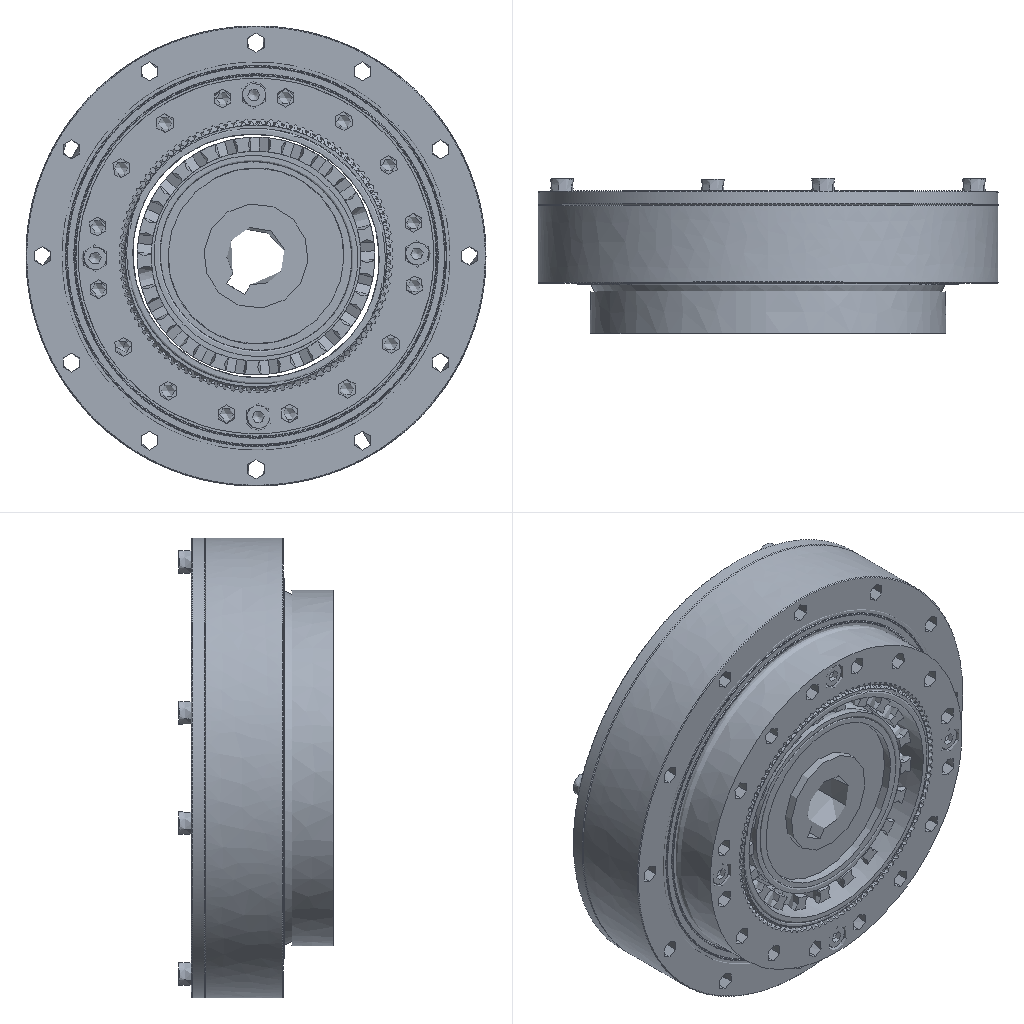Simulation study | ansys workbench
Set-up summary:
category,name,step,type,value,unit,region
solver,ansys_mapdl
solver,version,,,22.1
units,MPA,,stated
analysis,deck,,transient,transient
load_step,requested,,,1
analysis,nlgeom,,,True
mesh,nodes,,,225226
mesh,elements,,,154411
element_type,ANSYS 187 (type 1),,solid,2128
element_type,ANSYS 187 (type 2),,solid,3188
element_type,ANSYS 187 (type 3),,solid,1342
element_type,ANSYS 187 (type 4),,solid,24713
element_type,ANSYS 187 (type 5),,solid,9653
element_type,ANSYS 187 (type 6),,solid,9049
element_type,ANSYS 187 (type 7),,solid,3636
element_type,ANSYS 187 (type 8),,solid,2693
element_type,ANSYS 187 (type 9),,solid,23046
element_type,ANSYS 187 (type 10),,solid,29778
element_type,ANSYS 187 (type 11),,solid,1220
element_type,ANSYS 187 (type 12),,solid,1220
element_type,ANSYS 187 (type 13),,solid,1220
element_type,ANSYS 187 (type 14),,solid,1220
element_type,ANSYS 187 (type 15),,solid,1220
element_type,ANSYS 187 (type 16),,solid,1220
element_type,ANSYS 187 (type 17),,solid,1220
element_type,ANSYS 187 (type 18),,solid,1220
element_type,ANSYS 174 (type 19),,contact,1577
element_type,ANSYS 170 (type 20),,target,1577
element_type,ANSYS 174 (type 21),,contact,2406
element_type,ANSYS 170 (type 22),,target,2406
element_type,ANSYS 174 (type 23),,contact,561
element_type,ANSYS 170 (type 24),,target,561
element_type,ANSYS 174 (type 25),,contact,396
element_type,ANSYS 170 (type 26),,target,396
element_type,ANSYS 174 (type 27),,contact,1694
element_type,ANSYS 170 (type 28),,target,1694
element_type,ANSYS 174 (type 29),,contact,3067
element_type,ANSYS 170 (type 30),,target,3067
element_type,ANSYS 174 (type 31),,contact,124
element_type,ANSYS 170 (type 32),,target,124
element_type,ANSYS 174 (type 33),,contact,126
element_type,ANSYS 170 (type 34),,target,126
element_type,ANSYS 174 (type 35),,contact,122
element_type,ANSYS 170 (type 36),,target,122
element_type,ANSYS 174 (type 37),,contact,124
element_type,ANSYS 170 (type 38),,target,124
element_type,ANSYS 174 (type 39),,contact,363
element_type,ANSYS 170 (type 40),,target,363
element_type,ANSYS 174 (type 41),,contact,628
element_type,ANSYS 170 (type 42),,target,628
element_type,ANSYS 174 (type 43),,contact,912
element_type,ANSYS 170 (type 44),,target,912
element_type,ANSYS 174 (type 45),,contact,82
element_type,ANSYS 170 (type 46),,target,82
element_type,ANSYS 174 (type 47),,contact,84
element_type,ANSYS 170 (type 48),,target,84
element_type,ANSYS 174 (type 49),,contact,86
element_type,ANSYS 170 (type 50),,target,86
element_type,ANSYS 174 (type 51),,contact,82
element_type,ANSYS 170 (type 52),,target,82
element_type,ANSYS 174 (type 53),,contact,1510
element_type,ANSYS 170 (type 54),,target,1510
element_type,ANSYS 174 (type 55),,contact,308
element_type,ANSYS 170 (type 56),,target,308
element_type,ANSYS 174 (type 57),,contact,303
element_type,ANSYS 170 (type 58),,target,303
element_type,ANSYS 174 (type 59),,contact,303
element_type,ANSYS 170 (type 60),,target,303
element_type,ANSYS 174 (type 61),,contact,310
element_type,ANSYS 170 (type 62),,target,310
element_type,ANSYS 174 (type 63),,contact,236
element_type,ANSYS 170 (type 64),,target,236
element_type,ANSYS 174 (type 65),,contact,226
element_type,ANSYS 170 (type 66),,target,226
element_type,ANSYS 174 (type 67),,contact,234
element_type,ANSYS 170 (type 68),,target,234
element_type,ANSYS 174 (type 69),,contact,226
element_type,ANSYS 170 (type 70),,target,226
element_type,ANSYS 174 (type 71),,contact,3245
element_type,ANSYS 170 (type 72),,target,0
load,load commands in deck,,count,3
bc,support commands in deck,,count,1
named_set,_FIXEDSU,,component
material,1,,in results
material,2,,in results
material,3,,in results
material,4,,in results
material,5,,in results
material,6,,in results
material,7,,in results
material,8,,in results
material,9,,in results
material,10,,in results
material,11,,in results
material,12,,in results
material,13,,in results
material,14,,in results
material,15,,in results
material,16,,in results
material,17,,in results
material,18,,in results
check,setup vs results,,match,results also hold 0 node(s) and 1 element(s) the deck makes with ['EN']; those were not compared; 1 node(s) the solver created internally for pilot nodes (solve.out) are in the results only
Ansys APDL input file, long lists of numbers shortened:
/batch
/config,noeldb,1     ! force off writing results to database
*get,_wallstrt,active,,time,wall
! ANSYS input file written by Workbench version 2022 R1
! File used for geometry attach: F:\ansys（分析文件汇总)\齿轮减速机有限元分析\M6170-谐波齿轮减速机三维SW2014带参+MF1219218=100\谐波齿轮减速机.STEP
/title,wbnew--__ (B5)
! ****** Begin Custom Load Command Snippet ******
/COM, ACT Extensions:
/COM,     LSDYNA, 2021.1
/COM,
! ****** End   Custom Load Command Snippet ******
*DIM,_wb_ProjectScratch_dir,string,248
_wb_ProjectScratch_dir(1) = 'C:\Users\Administrator\AppData\Local\Temp\WB_Administrator_26020_2\_ProjectScratch\Scr0A8C\'
*DIM,_wb_SolverFiles_dir,string,248
_wb_SolverFiles_dir(1) = 'C:\Users\Administrator\AppData\Local\Temp\WB_Administrator_26020_2\wbnew_files\dp0\SYS\MECH\'
*DIM,_wb_userfiles_dir,string,248
_wb_userfiles_dir(1) = 'C:\Users\Administrator\AppData\Local\Temp\WB_Administrator_26020_2\wbnew_files\user_files\'
/com,--- Data in consistent NMM units. See Solving Units in the help system for more information.
/units,MPA
/nopr
/wb,file,start              !  signify a WB generated input file
/prep7
! Turn off shape checking because checks already performed inside WB mesher.
! See help system for more information.
SHPP,OFF,,NOWARN
/nolist
etcon,set             ! allow ANSYS to choose best KEYOP's for 180x elements, resets any applicable keyopt to MAPDL defaults
/com,*********** Nodes for the whole assembly ***********
nblock,3,,247747
(1i9,3e20.9e3)
    45460    -7.855159955E+00    -2.001121905E+01     1.580752509E+02
! (225224 more lines like these left out)
-1
/com,*********** Nodes for all Remote Points ***********
nblock,3
(1i9,3e20.9e3)
   273412    -7.293931818E+00    -4.673224382E+00     1.196122838E+02
-1
/wb,elem,start            !  set before creation of elements
/com,*********** Elements for Body 1 "____|__(____)|__-__1" ***********
et,1,187
eblock,19,solid,,2128
(19i9)
        1        1        1        1        0        0        0        0       10        0    34206    89365    89962    89993    89963    90422    93810    90424    90423
! (4255 more lines like these left out)
-1
/com,*********** Elements for Body 2 "____|__(____)|__-__2" ***********
et,2,187
eblock,19,solid,,3188
(19i9)
        2        2        2        2        0        0        0        0       10        0    70700   156902   157665   158100   158090   159082   163245   159086   159085
! (6375 more lines like these left out)
-1
/com,*********** Elements for Body 3 "____|_________|__(__)1" ***********
et,3,187
eblock,19,solid,,1342
(19i9)
        3        3        3        3        0        0        0        0       10        0    21122    65542    66163    65554    66140    66628    66692    66623    66627
! (2683 more lines like these left out)
-1
/com,*********** Elements for Body 4 "______|__________|__1" ***********
et,4,187
eblock,19,solid,,24713
(19i9)
        4        4        4        4        0        0        0        0       10        0    36334    99419    99428   101282   100310   132259   132316   132264   132262
! (49425 more lines like these left out)
-1
/com,*********** Elements for Body 5 "______|___________|__1" ***********
et,5,187
eblock,19,solid,,9653
(19i9)
        5        5        5        5        0        0        0        0       10        0    61047   141015   141186   141606   141558   154946   155797   154949   154948
! (19305 more lines like these left out)
-1
! (13 more sections like these left out)
/wb,elem,end               !  done creating elements
/com,*********** Send User Defined Coordinate System(s) ***********
csys,0
toffst,273.15,  ! Temperature offset from absolute zero
/com,*********** Set Reference Temperature ***********
tref,22.
/wb,mat,start              !  starting to send materials
/com,*********** Send Materials ***********
Temperature = 'TEMP' ! Temperature
MP,DENS,1,7.85e-09,	! tonne mm^-3
MP,ALPX,1,1.2e-05,	! C^-1
MP,C,1,434000000,	! mm^2 s^-2 C^-1
MP,KXX,1,60.5,	! tonne mm s^-3 C^-1
MP,RSVX,1,0.00017,	! ohm mm
MP,EX,1,200000,	! tonne s^-2 mm^-1
MP,NUXY,1,0.3,
MP,MURX,1,10000,
Temperature = 'TEMP' ! Temperature
MP,DENS,2,7.85e-09,	! tonne mm^-3
MP,ALPX,2,1.2e-05,	! C^-1
MP,C,2,434000000,	! mm^2 s^-2 C^-1
MP,KXX,2,60.5,	! tonne mm s^-3 C^-1
MP,RSVX,2,0.00017,	! ohm mm
MP,EX,2,200000,	! tonne s^-2 mm^-1
MP,NUXY,2,0.3,
MP,MURX,2,10000,
Temperature = 'TEMP' ! Temperature
MP,DENS,3,7.85e-09,	! tonne mm^-3
MP,ALPX,3,1.2e-05,	! C^-1
MP,C,3,434000000,	! mm^2 s^-2 C^-1
MP,KXX,3,60.5,	! tonne mm s^-3 C^-1
MP,RSVX,3,0.00017,	! ohm mm
MP,EX,3,200000,	! tonne s^-2 mm^-1
MP,NUXY,3,0.3,
MP,MURX,3,10000,
Temperature = 'TEMP' ! Temperature
MP,DENS,4,7.85e-09,	! tonne mm^-3
MP,ALPX,4,1.2e-05,	! C^-1
MP,C,4,434000000,	! mm^2 s^-2 C^-1
MP,KXX,4,60.5,	! tonne mm s^-3 C^-1
MP,RSVX,4,0.00017,	! ohm mm
MP,EX,4,200000,	! tonne s^-2 mm^-1
MP,NUXY,4,0.3,
MP,MURX,4,10000,
Temperature = 'TEMP' ! Temperature
MP,DENS,5,7.85e-09,	! tonne mm^-3
MP,ALPX,5,1.2e-05,	! C^-1
MP,C,5,434000000,	! mm^2 s^-2 C^-1
MP,KXX,5,60.5,	! tonne mm s^-3 C^-1
MP,RSVX,5,0.00017,	! ohm mm
MP,EX,5,200000,	! tonne s^-2 mm^-1
MP,NUXY,5,0.3,
MP,MURX,5,10000,
Temperature = 'TEMP' ! Temperature
MP,DENS,6,7.85e-09,	! tonne mm^-3
MP,ALPX,6,1.2e-05,	! C^-1
MP,C,6,434000000,	! mm^2 s^-2 C^-1
MP,KXX,6,60.5,	! tonne mm s^-3 C^-1
MP,RSVX,6,0.00017,	! ohm mm
MP,EX,6,200000,	! tonne s^-2 mm^-1
MP,NUXY,6,0.3,
MP,MURX,6,10000,
Temperature = 'TEMP' ! Temperature
MP,DENS,7,7.85e-09,	! tonne mm^-3
MP,ALPX,7,1.2e-05,	! C^-1
MP,C,7,434000000,	! mm^2 s^-2 C^-1
MP,KXX,7,60.5,	! tonne mm s^-3 C^-1
MP,RSVX,7,0.00017,	! ohm mm
MP,EX,7,200000,	! tonne s^-2 mm^-1
MP,NUXY,7,0.3,
MP,MURX,7,10000,
Temperature = 'TEMP' ! Temperature
MP,DENS,8,7.85e-09,	! tonne mm^-3
MP,ALPX,8,1.2e-05,	! C^-1
MP,C,8,434000000,	! mm^2 s^-2 C^-1
MP,KXX,8,60.5,	! tonne mm s^-3 C^-1
MP,RSVX,8,0.00017,	! ohm mm
MP,EX,8,200000,	! tonne s^-2 mm^-1
MP,NUXY,8,0.3,
MP,MURX,8,10000,
Temperature = 'TEMP' ! Temperature
MP,DENS,9,7.85e-09,	! tonne mm^-3
MP,ALPX,9,1.2e-05,	! C^-1
MP,C,9,434000000,	! mm^2 s^-2 C^-1
MP,KXX,9,60.5,	! tonne mm s^-3 C^-1
MP,RSVX,9,0.00017,	! ohm mm
MP,EX,9,200000,	! tonne s^-2 mm^-1
! (83 more lines like these left out)
/wb,mat,end                !  done sending materials
!************************* Model Summary ********************
!____|__(____)|__-__1,	结构钢,	matid,	1
!____|__(____)|__-__2,	结构钢,	matid,	2
!____|_________|__(__)1,	结构钢,	matid,	3
!______|__________|__1,	结构钢,	matid,	4
!______|___________|__1,	结构钢,	matid,	5
!______|__________|M4 ___1,	结构钢,	matid,	6
!______|___________|__(__)2,	结构钢,	matid,	7
!____|__-__2,	结构钢,	matid,	8
!__|__(__)1,	结构钢,	matid,	9
!__|__(__)4,	结构钢,	matid,	10
!socket head cap screw_iso_ISO 4762 M3 x 12 --- 12C|Hex,	结构钢,	matid,	11
!socket head cap screw_iso_ISO 4762 M3 x 12 --- 12C|Hex[2],	结构钢,	matid,	12
!socket head cap screw_iso_ISO 4762 M3 x 12 --- 12C|Hex[3],	结构钢,	matid,	13
!socket head cap screw_iso_ISO 4762 M3 x 12 --- 12C|Hex[4],	结构钢,	matid,	14
!socket head cap screw_iso_ISO 4762 M3 x 12 --- 12C|Hex[5],	结构钢,	matid,	15
!socket head cap screw_iso_ISO 4762 M3 x 12 --- 12C|Hex[6],	结构钢,	matid,	16
!socket head cap screw_iso_ISO 4762 M3 x 12 --- 12C|Hex[7],	结构钢,	matid,	17
!socket head cap screw_iso_ISO 4762 M3 x 12 --- 12C|Hex[8],	结构钢,	matid,	18
!************************* End Model Summary ********************
! get the diagonal of the bounding box. Needed later for other things
*get,_xmin,node,,mnloc,x
*get,_ymin,node,,mnloc,y
*get,_zmin,node,,mnloc,z
*get,_xmax,node,,mxloc,x
*get,_ymax,node,,mxloc,y
*get,_zmax,node,,mxloc,z
_ASMDIAG=(_xmax-_xmin)*(_xmax-_xmin)+(_ymax-_ymin)*(_ymax-_ymin)+(_zmax-_zmin)*(_zmax-_zmin)
_ASMDIAG=SQRT(_ASMDIAG)
/wb,contact,start          !  starting to send contact
/com,*********** Create Contact "接触区域 22" ***********
/com,            Real Constant Set For Above Contact Is 20 & 19
*set,tid,20
*set,cid,19
r,tid
r,cid
et,tid,170
et,cid,174
eblock,10,,,1195
(15i9)
   200887       20       20       20        0    89390    90167    89854    89854    90694    93366    89854    90692
! (1194 more lines like these left out)
-1
eblock,10,,,1195
(15i9)
   202082       19       19       19        0    89390    90167    89854    89854    90694    93366    89854    90692
! (1194 more lines like these left out)
-1
eblock,10,,,382
(15i9)
   203277       19       20       19        0    68935    69492    69369    69369    70292    72791    69369    70290
! (381 more lines like these left out)
-1
eblock,10,,,382
(15i9)
   203659       20       19       20        0    68935    69492    69369    69369    70292    72791    69369    70290
! (381 more lines like these left out)
-1
keyo,cid,8,2               ! auto create asymmetric contact (from Program Controlled setting)
keyo,cid,10,0              ! adjust contact stiffness each NR iteration (from Program Controlled setting)
keyo,cid,12,5              ! bonded always
keyo,cid,18,1              ! small sliding turned on by application
keyo,cid,2,0               ! augmented Lagrange (from Program Controlled setting)
keyo,cid,4,0               ! on Gauss point (from Program Controlled setting)
keyo,cid,9,1               ! ignore initial gaps/penetration
keyo,cid,7,0               ! No Prediction
rmod,tid,3,10.      ! FKN
rmod,tid,5,0.       ! ICONT
rmod,tid,6,0.       ! PINB
rmod,tid,10,0.      ! CNOF
rmod,tid,12,0.      ! FKT
rmod,tid,36,335     ! WB DSID
rmod,cid,3,10.      ! FKN
rmod,cid,5,0.       ! ICONT
rmod,cid,6,0.       ! PINB
rmod,cid,10,0.      ! CNOF
rmod,cid,12,0.      ! FKT
rmod,cid,36,335     ! WB DSID
/com,*********** Create Contact "接触区域 44" ***********
/com,            Real Constant Set For Above Contact Is 22 & 21
*set,tid,22
*set,cid,21
r,tid
r,cid
et,tid,170
et,cid,174
eblock,10,,,1924
(15i9)
   204041       22       22       22        0   156847   157305   158010   158010   158679   162016   158010   158681
! (1923 more lines like these left out)
-1
eblock,10,,,1924
(15i9)
   205965       21       21       21        0   156847   157305   158010   158010   158679   162016   158010   158681
! (1923 more lines like these left out)
-1
eblock,10,,,482
(15i9)
   207889       21       22       21        0   224115   217811   225802   225802   236699   236706   225802   269653
! (481 more lines like these left out)
-1
eblock,10,,,482
(15i9)
   208371       22       21       22        0   224115   217811   225802   225802   236699   236706   225802   269653
! (481 more lines like these left out)
-1
keyo,cid,8,2               ! auto create asymmetric contact (from Program Controlled setting)
keyo,cid,10,0              ! adjust contact stiffness each NR iteration (from Program Controlled setting)
keyo,cid,12,5              ! bonded always
keyo,cid,18,1              ! small sliding turned on by application
keyo,cid,2,0               ! augmented Lagrange (from Program Controlled setting)
keyo,cid,4,0               ! on Gauss point (from Program Controlled setting)
keyo,cid,9,1               ! ignore initial gaps/penetration
keyo,cid,7,0               ! No Prediction
rmod,tid,3,10.      ! FKN
rmod,tid,5,0.       ! ICONT
rmod,tid,6,0.       ! PINB
rmod,tid,10,0.      ! CNOF
rmod,tid,12,0.      ! FKT
rmod,tid,36,401     ! WB DSID
rmod,cid,3,10.      ! FKN
rmod,cid,5,0.       ! ICONT
rmod,cid,6,0.       ! PINB
rmod,cid,10,0.      ! CNOF
rmod,cid,12,0.      ! FKT
rmod,cid,36,401     ! WB DSID
/com,*********** Create Contact "接触区域 66" ***********
/com,            Real Constant Set For Above Contact Is 24 & 23
*set,tid,24
*set,cid,23
r,tid
r,cid
et,tid,170
et,cid,174
eblock,10,,,208
(15i9)
   208853       24       24       24        0    95023    97163    97175    97175   107749   120331    97175   107750
! (207 more lines like these left out)
-1
eblock,10,,,208
(15i9)
   209061       23       23       23        0    95023    97163    97175    97175   107749   120331    97175   107750
! (207 more lines like these left out)
-1
eblock,10,,,353
(15i9)
   209269       23       24       23        0   138718   139115   138739   138739   142500   142663   138739   142498
! (352 more lines like these left out)
-1
eblock,10,,,353
(15i9)
   209622       24       23       24        0   138718   139115   138739   138739   142500   142663   138739   142498
! (352 more lines like these left out)
-1
keyo,cid,8,2               ! auto create asymmetric contact (from Program Controlled setting)
keyo,cid,10,0              ! adjust contact stiffness each NR iteration (from Program Controlled setting)
keyo,cid,12,5              ! bonded always
keyo,cid,18,1              ! small sliding turned on by application
keyo,cid,2,0               ! augmented Lagrange (from Program Controlled setting)
keyo,cid,4,0               ! on Gauss point (from Program Controlled setting)
keyo,cid,9,1               ! ignore initial gaps/penetration
keyo,cid,7,0               ! No Prediction
rmod,tid,3,10.      ! FKN
rmod,tid,5,0.       ! ICONT
rmod,tid,6,0.       ! PINB
rmod,tid,10,0.      ! CNOF
rmod,tid,12,0.      ! FKT
rmod,tid,36,467     ! WB DSID
rmod,cid,3,10.      ! FKN
rmod,cid,5,0.       ! ICONT
rmod,cid,6,0.       ! PINB
rmod,cid,10,0.      ! CNOF
rmod,cid,12,0.      ! FKT
rmod,cid,36,467     ! WB DSID
/com,*********** Create Contact "接触区域 67" ***********
/com,            Real Constant Set For Above Contact Is 26 & 25
*set,tid,26
*set,cid,25
r,tid
r,cid
et,tid,170
et,cid,174
eblock,10,,,210
(15i9)
   209975       26       26       26        0    94982    97157    95268    95268   107376   110221    95268   107375
! (209 more lines like these left out)
-1
eblock,10,,,210
(15i9)
   210185       25       25       25        0    94982    97157    95268    95268   107376   110221    95268   107375
! (209 more lines like these left out)
-1
eblock,10,,,186
(15i9)
   210395       25       26       25        0    74267    74881    74269    74269    79156    79168    74269    79153
! (185 more lines like these left out)
-1
eblock,10,,,186
(15i9)
   210581       26       25       26        0    74267    74881    74269    74269    79156    79168    74269    79153
! (185 more lines like these left out)
-1
keyo,cid,8,2               ! auto create asymmetric contact (from Program Controlled setting)
keyo,cid,10,0              ! adjust contact stiffness each NR iteration (from Program Controlled setting)
keyo,cid,12,5              ! bonded always
keyo,cid,18,1              ! small sliding turned on by application
keyo,cid,2,0               ! augmented Lagrange (from Program Controlled setting)
keyo,cid,4,0               ! on Gauss point (from Program Controlled setting)
keyo,cid,9,1               ! ignore initial gaps/penetration
keyo,cid,7,0               ! No Prediction
rmod,tid,3,10.      ! FKN
rmod,tid,5,0.       ! ICONT
rmod,tid,6,0.       ! PINB
rmod,tid,10,0.      ! CNOF
rmod,tid,12,0.      ! FKT
rmod,tid,36,470     ! WB DSID
rmod,cid,3,10.      ! FKN
rmod,cid,5,0.       ! ICONT
rmod,cid,6,0.       ! PINB
rmod,cid,10,0.      ! CNOF
rmod,cid,12,0.      ! FKT
rmod,cid,36,470     ! WB DSID
/com,*********** Create Contact "接触区域 68" ***********
/com,            Real Constant Set For Above Contact Is 28 & 27
*set,tid,28
*set,cid,27
r,tid
r,cid
et,tid,170
et,cid,174
eblock,10,,,682
(15i9)
   210767       28       28       28        0    94958    98011    98194    98194   107215   123362    98194   107216
! (681 more lines like these left out)
-1
eblock,10,,,682
(15i9)
   211449       27       27       27        0    94958    98011    98194    98194   107215   123362    98194   107216
! (681 more lines like these left out)
-1
eblock,10,,,1012
(15i9)
   212131       27       28       27        0   164144   164083   164928   164928   166746   166750   164928   167137
! (1011 more lines like these left out)
-1
eblock,10,,,1012
(15i9)
   213143       28       27       28        0   164144   164083   164928   164928   166746   166750   164928   167137
! (1011 more lines like these left out)
-1
keyo,cid,8,2               ! auto create asymmetric contact (from Program Controlled setting)
keyo,cid,10,0              ! adjust contact stiffness each NR iteration (from Program Controlled setting)
keyo,cid,12,5              ! bonded always
keyo,cid,18,1              ! small sliding turned on by application
keyo,cid,2,0               ! augmented Lagrange (from Program Controlled setting)
keyo,cid,4,0               ! on Gauss point (from Program Controlled setting)
keyo,cid,9,1               ! ignore initial gaps/penetration
keyo,cid,7,0               ! No Prediction
rmod,tid,3,10.      ! FKN
rmod,tid,5,0.       ! ICONT
rmod,tid,6,0.       ! PINB
rmod,tid,10,0.      ! CNOF
rmod,tid,12,0.      ! FKT
rmod,tid,36,473     ! WB DSID
rmod,cid,3,10.      ! FKN
rmod,cid,5,0.       ! ICONT
rmod,cid,6,0.       ! PINB
rmod,cid,10,0.      ! CNOF
rmod,cid,12,0.      ! FKT
rmod,cid,36,473     ! WB DSID
! (21 more sections like these left out)
/wb,contact,end            !  done creating contacts
/golist
/wb,load,start             !  starting to send loads
/com,*********** Fixed Supports ***********
CMBLOCK,_FIXEDSU,NODE,    17247
(8i10)
     45465     45466     45467     45468     45469     45470     45510     45511
! (2155 more lines like these left out)
cmsel,s,_FIXEDSU
d,all,all
nsel,all
/com,*********** Create Remote Point "内部远程点" ***********
! -------- Remote Point Used by "力矩" --------
*set,tid,72
*set,cid,71
et,cid,174
et,tid,170
keyo,tid,2,1               ! Don't fix the pilot node
keyo,tid,4,0               ! Activate all DOF's due to large deformation
keyo,cid,12,5              ! Bonded Contact
keyo,cid,4,1               ! Deformable RBE3 style load
keyo,cid,2,2               ! MPC style contact
eblock,10,,,3245
(15i9)
   233067       71       71       71        0   224115   217811   225802   225802   236699   236706   225802   269653
! (3244 more lines like these left out)
-1
*set,_npilot,273412
_npilot943=_npilot
type,tid
mat ,cid
real,cid
tshape,pilo
en,236312,_npilot
tshape
/com,*********** Construct Moment Using Remote Attachment ***********
/gst,on,on
fini
*get,_numnode,node,0,count
*get,_numelem,elem,0,count
*get, _MAXELEMNUM, elem, 0, NUM, MAX
*get, _MAXNODENUM, node, 0, NUM, MAX
*get, _MAXELEMTYPE, etyp, 0, NUM, MAX
*get, _MAXREALCONST, real, 0, NUM, MAX
/go
/wb,load,end               !  done creating loads
/com,--- Number of total nodes = %_numnode%
/com,--- Number of contact elements = 35425
/com,--- Number of spring elements = 0
/com,--- Number of bearing elements = 0
/com,--- Number of solid elements = 118986
/com,--- Number of condensed parts = 0
/com,--- Number of total elements = %_numelem%
*get,_wallbsol,active,,time,wall
/com,****************************************************************************
/com,*************************    SOLUTION       ********************************
/com,****************************************************************************
/solu
antype,4                   ! transient analysis
nlgeom,on                  ! Turn on Large Deformation Effects
kbc,1                      ! stepped BC's
_thickRatio=0.722   ! Ratio of thick parts in the model
eqsl,pcg,1e-8,,,,,,1
cntr,print,1               ! print out contact info and also make no initial contact an error
dmpoption,emat,no             ! Don't combine emat file for DANSYS
dmpoption,esav,no             ! Don't combine esav file for DANSYS
trnopt,full,,,,,hht        ! HHT time integration method
tintp, mosp			! Choose transient integration settings for moderate speed application
nldiag,cont,iter           ! print out contact info each equilibrium iteration
rescontrol,define,last,last,,dele	   ! Program Controlled
/com,****************************************************
/com,******************* SOLVE FOR LS 1 OF 1 ****************
nsel,s,node,,273412
f,all,mx,0.
f,all,my,50000.
f,all,mz,0.
nsel,all
/nopr
/gopr
autots,on                   ! User turned on automatic time stepping
deltim,1,1,1,OFF
time,1.
timint,on                  ! Turn on time integration effects
outres,erase
outres,all,none
outres,nsol,all,
outres,rsol,all
outres,eangl,all
outres,etmp,all
outres,veng,all
outres,strs,all,
outres,epel,all,
outres,eppl,all,
outres,cont,all,
outres,v,all,
outres,a,all,
! *********** WB SOLVE COMMAND ***********
! check interactive state
*get,ANSINTER_,active,,int
*if,ANSINTER_,ne,0,then
/eof
*endif
solve
/com *************** Write FE CONNECTORS *********
CEWRITE,file,ce,,INTE
/com,****************************************************
/com,*************** FINISHED SOLVE FOR LS 1 *************
*get,_wallasol,active,,time,wall
/nopr
*get,_numnode,node,0,count
*get,_numelem,elem,0,count
*get, _MAXELEMNUM, elem, 0, NUM, MAX
*get, _MAXNODENUM, node, 0, NUM, MAX,,,INTERNAL
*get, _MAXELEMTYPE, etyp, 0, NUM, MAX
*get, _MAXREALCONST, real, 0, NUM, MAX
/gopr
*get,_PCGITER,active,,solu,cgiter
/post1
xmlo,ENCODING,ISO-8859-1
xmlo,parm
/xml,parm,xml
fini
/gopr
*get,_walldone,active,,time,wall
_preptime=(_wallbsol-_wallstrt)*3600
_solvtime=(_wallasol-_wallbsol)*3600
_posttime=(_walldone-_wallasol)*3600
_totaltim=(_walldone-_wallstrt)*3600
*get,_dlbratio,active,0,solu,dlbr
*get,_combtime,active,0,solu,comb
*get,_ssmode,active,0,solu,ssmm
*get,_ndofs,active,0,solu,ndof
*get,_sol_end_time,active,0,set,time
*if,_sol_end_time,eq,1.,then
/fclean				!clean distributed files
*endif
/com,--- Total number of nodes = %_numnode%
/com,--- Total number of elements = %_numelem%
/com,--- Element load balance ratio = %_dlbratio%
/com,--- Time to combine distributed files = %_combtime%
/com,--- Sparse memory mode = %_ssmode%
/com,--- Number of DOF = %_ndofs%
/wb,file,end               ! done with WB generated input
Results summary:
result,analysis,,,static
result,last_loadstep,,,1
result,primary field,,,displacement
result,reaction total,1,FX,-0.0,N
result,reaction total,1,FY,0.0,N
result,reaction total,1,FZ,-1e-06,N
result,mass,,,0.001212,"NMM: mm, ton, N, s, mV, mA, degC"